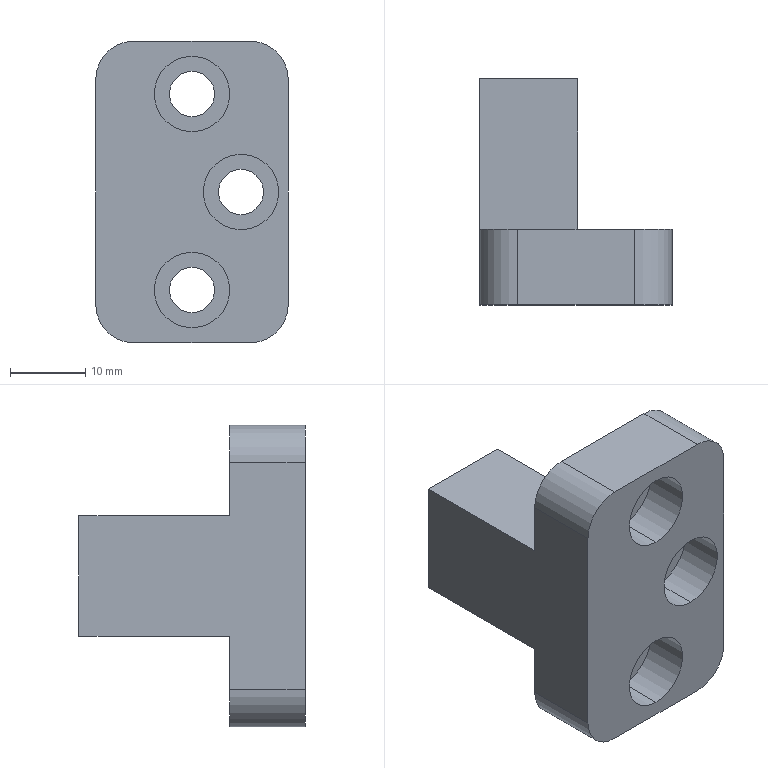Part | STEP file | 1 solid | 29 faces | box 25.5 x 30 x 40 mm | volume 12392 mm3 | cylinder 16 | plane 13 | commonest cylinder face diameters 10 x10 6 x6